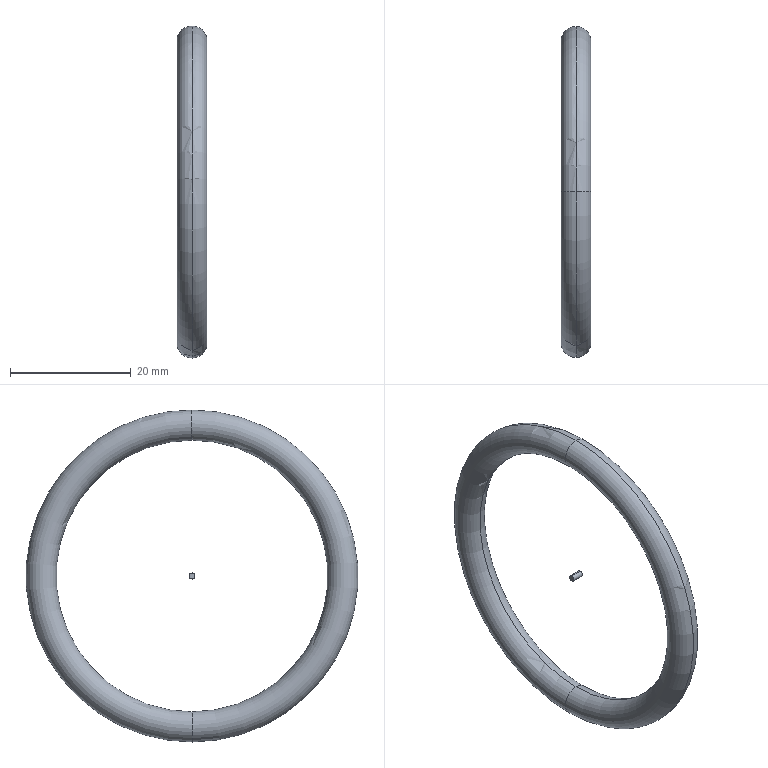Part | STEP file | Tension spring | 2 solids | 12 faces | box 5 x 55 x 55 mm | volume 1304 mm3 | torus 8 | cylinder 2 | plane 2 | commonest cylinder face diameters 1 x2
STEP:
#1=CARTESIAN_POINT('',(0.,0.,0.));
#2=DIRECTION('',(0.,0.,1.));
#3=DIRECTION('',(1.,0.,0.));
#4=AXIS2_PLACEMENT_3D('',#1,#2,#3);
#5=CARTESIAN_POINT('',(0.,0.,2.5));
#6=VERTEX_POINT('',#5);
#7=CARTESIAN_POINT('',(0.,0.,-2.5));
#8=VERTEX_POINT('',#7);
#9=CARTESIAN_POINT('',(0.,0.,0.));
#10=DIRECTION('',(0.,1.,0.));
#11=DIRECTION('',(0.,0.,1.));
#12=AXIS2_PLACEMENT_3D('',#9,#10,#11);
#13=CIRCLE('',#12,2.5);
#14=CARTESIAN_POINT('',(0.,0.,-25.));
#15=DIRECTION('',(1.,0.,0.));
#16=DIRECTION('',(0.,0.,-1.));
#17=AXIS2_PLACEMENT_3D('',#14,#15,#16);
#18=TOROIDAL_SURFACE('',#17,25.,2.5);
#19=CARTESIAN_POINT('',(3.142,0.));
#20=DIRECTION('',(0.,1.));
#21=VECTOR('',#20,1.);
#22=LINE('',#19,#21);
#23=(GEOMETRIC_REPRESENTATION_CONTEXT(2)PARAMETRIC_REPRESENTATION_CONTEXT()REPRESENTATION_CONTEXT('',''));
#24=DEFINITIONAL_REPRESENTATION('',(#22),#23);
#25=PCURVE('',#18,#24);
#26=CARTESIAN_POINT('',(0.,0.,-25.));
#27=DIRECTION('',(1.,0.,0.));
#28=DIRECTION('',(0.,0.,-1.));
#29=AXIS2_PLACEMENT_3D('',#26,#27,#28);
#30=TOROIDAL_SURFACE('',#29,25.,2.5);
#31=CARTESIAN_POINT('',(3.142,0.));
#32=DIRECTION('',(0.,1.));
#33=VECTOR('',#32,1.);
#34=LINE('',#31,#33);
#35=(GEOMETRIC_REPRESENTATION_CONTEXT(2)PARAMETRIC_REPRESENTATION_CONTEXT()REPRESENTATION_CONTEXT('',''));
#36=DEFINITIONAL_REPRESENTATION('',(#34),#35);
#37=PCURVE('',#30,#36);
#38=SURFACE_CURVE('',#13,(#25,#37),.PCURVE_S1.);
#39=EDGE_CURVE('',#6,#8,#38,.T.);
#40=ORIENTED_EDGE('',*,*,#39,.F.);
#41=CARTESIAN_POINT('',(0.,0.,-52.5));
#42=VERTEX_POINT('',#41);
#43=CARTESIAN_POINT('',(0.,0.,-25.));
#44=DIRECTION('',(1.,0.,0.));
#45=DIRECTION('',(0.,0.,-1.));
#46=AXIS2_PLACEMENT_3D('',#43,#44,#45);
#47=CIRCLE('',#46,27.5);
#48=CARTESIAN_POINT('',(0.,0.));
#49=DIRECTION('',(1.,0.));
#50=VECTOR('',#49,1.);
#51=LINE('',#48,#50);
#52=(GEOMETRIC_REPRESENTATION_CONTEXT(2)PARAMETRIC_REPRESENTATION_CONTEXT()REPRESENTATION_CONTEXT('',''));
#53=DEFINITIONAL_REPRESENTATION('',(#51),#52);
#54=PCURVE('',#18,#53);
#55=CARTESIAN_POINT('',(0.,0.,-25.));
#56=DIRECTION('',(1.,0.,0.));
#57=DIRECTION('',(0.,0.,-1.));
#58=AXIS2_PLACEMENT_3D('',#55,#56,#57);
#59=TOROIDAL_SURFACE('',#58,25.,2.5);
#60=CARTESIAN_POINT('',(0.,6.283));
#61=DIRECTION('',(1.,0.));
#62=VECTOR('',#61,1.);
#63=LINE('',#60,#62);
#64=(GEOMETRIC_REPRESENTATION_CONTEXT(2)PARAMETRIC_REPRESENTATION_CONTEXT()REPRESENTATION_CONTEXT('',''));
#65=DEFINITIONAL_REPRESENTATION('',(#63),#64);
#66=PCURVE('',#59,#65);
#67=SURFACE_CURVE('',#47,(#54,#66),.PCURVE_S1.);
#68=EDGE_CURVE('',#6,#42,#67,.T.);
#69=ORIENTED_EDGE('',*,*,#68,.T.);
#70=CARTESIAN_POINT('',(0.,0.,-47.5));
#71=VERTEX_POINT('',#70);
#72=CARTESIAN_POINT('',(0.,0.,-50.));
#73=DIRECTION('',(0.,-1.,0.));
#74=DIRECTION('',(0.,0.,-1.));
#75=AXIS2_PLACEMENT_3D('',#72,#73,#74);
#76=CIRCLE('',#75,2.5);
#77=CARTESIAN_POINT('',(6.283,0.));
#78=DIRECTION('',(0.,1.));
#79=VECTOR('',#78,1.);
#80=LINE('',#77,#79);
#81=(GEOMETRIC_REPRESENTATION_CONTEXT(2)PARAMETRIC_REPRESENTATION_CONTEXT()REPRESENTATION_CONTEXT('',''));
#82=DEFINITIONAL_REPRESENTATION('',(#80),#81);
#83=PCURVE('',#18,#82);
#84=CARTESIAN_POINT('',(0.,0.));
#85=DIRECTION('',(0.,1.));
#86=VECTOR('',#85,1.);
#87=LINE('',#84,#86);
#88=(GEOMETRIC_REPRESENTATION_CONTEXT(2)PARAMETRIC_REPRESENTATION_CONTEXT()REPRESENTATION_CONTEXT('',''));
#89=DEFINITIONAL_REPRESENTATION('',(#87),#88);
#90=PCURVE('',#30,#89);
#91=SURFACE_CURVE('',#76,(#83,#90),.PCURVE_S1.);
#92=EDGE_CURVE('',#42,#71,#91,.T.);
#93=ORIENTED_EDGE('',*,*,#92,.T.);
#94=CARTESIAN_POINT('',(0.,0.,-25.));
#95=DIRECTION('',(1.,0.,0.));
#96=DIRECTION('',(0.,0.,-1.));
#97=AXIS2_PLACEMENT_3D('',#94,#95,#96);
#98=CIRCLE('',#97,22.5);
#99=CARTESIAN_POINT('',(0.,3.142));
#100=DIRECTION('',(1.,0.));
#101=VECTOR('',#100,1.);
#102=LINE('',#99,#101);
#103=(GEOMETRIC_REPRESENTATION_CONTEXT(2)PARAMETRIC_REPRESENTATION_CONTEXT()REPRESENTATION_CONTEXT('',''));
#104=DEFINITIONAL_REPRESENTATION('',(#102),#103);
#105=PCURVE('',#18,#104);
#106=CARTESIAN_POINT('',(0.,3.142));
#107=DIRECTION('',(1.,0.));
#108=VECTOR('',#107,1.);
#109=LINE('',#106,#108);
#110=(GEOMETRIC_REPRESENTATION_CONTEXT(2)PARAMETRIC_REPRESENTATION_CONTEXT()REPRESENTATION_CONTEXT('',''));
#111=DEFINITIONAL_REPRESENTATION('',(#109),#110);
#112=PCURVE('',#59,#111);
#113=SURFACE_CURVE('',#98,(#105,#112),.PCURVE_S1.);
#114=EDGE_CURVE('',#8,#71,#113,.T.);
#115=ORIENTED_EDGE('',*,*,#114,.F.);
#116=EDGE_LOOP('',(#40,#69,#93,#115));
#117=FACE_BOUND('',#116,.T.);
#118=ADVANCED_FACE('',(#117),#18,.T.);
#119=ORIENTED_EDGE('',*,*,#92,.F.);
#120=CARTESIAN_POINT('',(0.,0.,-25.));
#121=DIRECTION('',(1.,0.,0.));
#122=DIRECTION('',(0.,0.,-1.));
#123=AXIS2_PLACEMENT_3D('',#120,#121,#122);
#124=CIRCLE('',#123,27.5);
#125=CARTESIAN_POINT('',(0.,0.));
#126=DIRECTION('',(1.,0.));
#127=VECTOR('',#126,1.);
#128=LINE('',#125,#127);
#129=(GEOMETRIC_REPRESENTATION_CONTEXT(2)PARAMETRIC_REPRESENTATION_CONTEXT()REPRESENTATION_CONTEXT('',''));
#130=DEFINITIONAL_REPRESENTATION('',(#128),#129);
#131=PCURVE('',#30,#130);
#132=CARTESIAN_POINT('',(0.,0.,-25.));
#133=DIRECTION('',(1.,0.,0.));
#134=DIRECTION('',(0.,0.,-1.));
#135=AXIS2_PLACEMENT_3D('',#132,#133,#134);
#136=TOROIDAL_SURFACE('',#135,25.,2.5);
#137=CARTESIAN_POINT('',(0.,6.283));
#138=DIRECTION('',(1.,0.));
#139=VECTOR('',#138,1.);
#140=LINE('',#137,#139);
#141=(GEOMETRIC_REPRESENTATION_CONTEXT(2)PARAMETRIC_REPRESENTATION_CONTEXT()REPRESENTATION_CONTEXT('',''));
#142=DEFINITIONAL_REPRESENTATION('',(#140),#141);
#143=PCURVE('',#136,#142);
#144=SURFACE_CURVE('',#124,(#131,#143),.PCURVE_S1.);
#145=EDGE_CURVE('',#42,#6,#144,.T.);
#146=ORIENTED_EDGE('',*,*,#145,.T.);
#147=ORIENTED_EDGE('',*,*,#39,.T.);
#148=CARTESIAN_POINT('',(0.,0.,-25.));
#149=DIRECTION('',(1.,0.,0.));
#150=DIRECTION('',(0.,0.,-1.));
#151=AXIS2_PLACEMENT_3D('',#148,#149,#150);
#152=CIRCLE('',#151,22.5);
#153=CARTESIAN_POINT('',(0.,3.142));
#154=DIRECTION('',(1.,0.));
#155=VECTOR('',#154,1.);
#156=LINE('',#153,#155);
#157=(GEOMETRIC_REPRESENTATION_CONTEXT(2)PARAMETRIC_REPRESENTATION_CONTEXT()REPRESENTATION_CONTEXT('',''));
#158=DEFINITIONAL_REPRESENTATION('',(#156),#157);
#159=PCURVE('',#30,#158);
#160=CARTESIAN_POINT('',(0.,3.142));
#161=DIRECTION('',(1.,0.));
#162=VECTOR('',#161,1.);
#163=LINE('',#160,#162);
#164=(GEOMETRIC_REPRESENTATION_CONTEXT(2)PARAMETRIC_REPRESENTATION_CONTEXT()REPRESENTATION_CONTEXT('',''));
#165=DEFINITIONAL_REPRESENTATION('',(#163),#164);
#166=PCURVE('',#136,#165);
#167=SURFACE_CURVE('',#152,(#159,#166),.PCURVE_S1.);
#168=EDGE_CURVE('',#71,#8,#167,.T.);
#169=ORIENTED_EDGE('',*,*,#168,.F.);
#170=EDGE_LOOP('',(#119,#146,#147,#169));
#171=FACE_BOUND('',#170,.T.);
#172=ADVANCED_FACE('',(#171),#30,.T.);
#173=ORIENTED_EDGE('',*,*,#145,.F.);
#174=CARTESIAN_POINT('',(0.,0.,-50.));
#175=DIRECTION('',(0.,-1.,0.));
#176=DIRECTION('',(0.,0.,-1.));
#177=AXIS2_PLACEMENT_3D('',#174,#175,#176);
#178=CIRCLE('',#177,2.5);
#179=CARTESIAN_POINT('',(0.,0.));
#180=DIRECTION('',(0.,1.));
#181=VECTOR('',#180,1.);
#182=LINE('',#179,#181);
#183=(GEOMETRIC_REPRESENTATION_CONTEXT(2)PARAMETRIC_REPRESENTATION_CONTEXT()REPRESENTATION_CONTEXT('',''));
#184=DEFINITIONAL_REPRESENTATION('',(#182),#183);
#185=PCURVE('',#136,#184);
#186=CARTESIAN_POINT('',(6.283,0.));
#187=DIRECTION('',(0.,1.));
#188=VECTOR('',#187,1.);
#189=LINE('',#186,#188);
#190=(GEOMETRIC_REPRESENTATION_CONTEXT(2)PARAMETRIC_REPRESENTATION_CONTEXT()REPRESENTATION_CONTEXT('',''));
#191=DEFINITIONAL_REPRESENTATION('',(#189),#190);
#192=PCURVE('',#59,#191);
#193=SURFACE_CURVE('',#178,(#185,#192),.PCURVE_S1.);
#194=EDGE_CURVE('',#71,#42,#193,.T.);
#195=ORIENTED_EDGE('',*,*,#194,.F.);
#196=ORIENTED_EDGE('',*,*,#168,.T.);
#197=CARTESIAN_POINT('',(0.,0.,0.));
#198=DIRECTION('',(0.,1.,0.));
#199=DIRECTION('',(0.,0.,1.));
#200=AXIS2_PLACEMENT_3D('',#197,#198,#199);
#201=CIRCLE('',#200,2.5);
#202=CARTESIAN_POINT('',(3.142,0.));
#203=DIRECTION('',(0.,1.));
#204=VECTOR('',#203,1.);
#205=LINE('',#202,#204);
#206=(GEOMETRIC_REPRESENTATION_CONTEXT(2)PARAMETRIC_REPRESENTATION_CONTEXT()REPRESENTATION_CONTEXT('',''));
#207=DEFINITIONAL_REPRESENTATION('',(#205),#206);
#208=PCURVE('',#136,#207);
#209=CARTESIAN_POINT('',(3.142,0.));
#210=DIRECTION('',(0.,1.));
#211=VECTOR('',#210,1.);
#212=LINE('',#209,#211);
#213=(GEOMETRIC_REPRESENTATION_CONTEXT(2)PARAMETRIC_REPRESENTATION_CONTEXT()REPRESENTATION_CONTEXT('',''));
#214=DEFINITIONAL_REPRESENTATION('',(#212),#213);
#215=PCURVE('',#59,#214);
#216=SURFACE_CURVE('',#201,(#208,#215),.PCURVE_S1.);
#217=EDGE_CURVE('',#8,#6,#216,.T.);
#218=ORIENTED_EDGE('',*,*,#217,.T.);
#219=EDGE_LOOP('',(#173,#195,#196,#218));
#220=FACE_BOUND('',#219,.T.);
#221=ADVANCED_FACE('',(#220),#136,.T.);
#222=ORIENTED_EDGE('',*,*,#68,.F.);
#223=ORIENTED_EDGE('',*,*,#217,.F.);
#224=ORIENTED_EDGE('',*,*,#114,.T.);
#225=ORIENTED_EDGE('',*,*,#194,.T.);
#226=EDGE_LOOP('',(#222,#223,#224,#225));
#227=FACE_BOUND('',#226,.T.);
#228=ADVANCED_FACE('',(#227),#59,.T.);
#229=CLOSED_SHELL('',(#118,#172,#221,#228));
#230=CARTESIAN_POINT('',(0.,0.,-48.1));
#231=VERTEX_POINT('',#230);
#232=CARTESIAN_POINT('',(0.,0.,-1.9));
#233=VERTEX_POINT('',#232);
#234=CARTESIAN_POINT('',(0.,0.,-25.));
#235=DIRECTION('',(1.,0.,0.));
#236=DIRECTION('',(0.,0.,-1.));
#237=AXIS2_PLACEMENT_3D('',#234,#235,#236);
#238=CIRCLE('',#237,23.1);
#239=CARTESIAN_POINT('',(0.,0.,-25.));
#240=DIRECTION('',(1.,0.,0.));
#241=DIRECTION('',(0.,0.,-1.));
#242=AXIS2_PLACEMENT_3D('',#239,#240,#241);
#243=TOROIDAL_SURFACE('',#242,25.,1.9);
#244=CARTESIAN_POINT('',(0.,3.142));
#245=DIRECTION('',(1.,0.));
#246=VECTOR('',#245,1.);
#247=LINE('',#244,#246);
#248=(GEOMETRIC_REPRESENTATION_CONTEXT(2)PARAMETRIC_REPRESENTATION_CONTEXT()REPRESENTATION_CONTEXT('',''));
#249=DEFINITIONAL_REPRESENTATION('',(#247),#248);
#250=PCURVE('',#243,#249);
#251=CARTESIAN_POINT('',(0.,0.,-25.));
#252=DIRECTION('',(1.,0.,0.));
#253=DIRECTION('',(0.,0.,-1.));
#254=AXIS2_PLACEMENT_3D('',#251,#252,#253);
#255=TOROIDAL_SURFACE('',#254,25.,1.9);
#256=CARTESIAN_POINT('',(0.,3.142));
#257=DIRECTION('',(1.,0.));
#258=VECTOR('',#257,1.);
#259=LINE('',#256,#258);
#260=(GEOMETRIC_REPRESENTATION_CONTEXT(2)PARAMETRIC_REPRESENTATION_CONTEXT()REPRESENTATION_CONTEXT('',''));
#261=DEFINITIONAL_REPRESENTATION('',(#259),#260);
#262=PCURVE('',#255,#261);
#263=SURFACE_CURVE('',#238,(#250,#262),.PCURVE_S1.);
#264=EDGE_CURVE('',#231,#233,#263,.T.);
#265=ORIENTED_EDGE('',*,*,#264,.T.);
#266=CARTESIAN_POINT('',(0.,0.,1.9));
#267=VERTEX_POINT('',#266);
#268=CARTESIAN_POINT('',(0.,0.,0.));
#269=DIRECTION('',(0.,1.,0.));
#270=DIRECTION('',(0.,0.,1.));
#271=AXIS2_PLACEMENT_3D('',#268,#269,#270);
#272=CIRCLE('',#271,1.9);
#273=CARTESIAN_POINT('',(3.142,0.));
#274=DIRECTION('',(0.,1.));
#275=VECTOR('',#274,1.);
#276=LINE('',#273,#275);
#277=(GEOMETRIC_REPRESENTATION_CONTEXT(2)PARAMETRIC_REPRESENTATION_CONTEXT()REPRESENTATION_CONTEXT('',''));
#278=DEFINITIONAL_REPRESENTATION('',(#276),#277);
#279=PCURVE('',#243,#278);
#280=CARTESIAN_POINT('',(0.,0.,-25.));
#281=DIRECTION('',(1.,0.,0.));
#282=DIRECTION('',(0.,0.,-1.));
#283=AXIS2_PLACEMENT_3D('',#280,#281,#282);
#284=TOROIDAL_SURFACE('',#283,25.,1.9);
#285=CARTESIAN_POINT('',(3.142,0.));
#286=DIRECTION('',(0.,1.));
#287=VECTOR('',#286,1.);
#288=LINE('',#285,#287);
#289=(GEOMETRIC_REPRESENTATION_CONTEXT(2)PARAMETRIC_REPRESENTATION_CONTEXT()REPRESENTATION_CONTEXT('',''));
#290=DEFINITIONAL_REPRESENTATION('',(#288),#289);
#291=PCURVE('',#284,#290);
#292=SURFACE_CURVE('',#272,(#279,#291),.PCURVE_S1.);
#293=EDGE_CURVE('',#233,#267,#292,.T.);
#294=ORIENTED_EDGE('',*,*,#293,.T.);
#295=CARTESIAN_POINT('',(0.,0.,-51.9));
#296=VERTEX_POINT('',#295);
#297=CARTESIAN_POINT('',(0.,0.,-25.));
#298=DIRECTION('',(1.,0.,0.));
#299=DIRECTION('',(0.,0.,-1.));
#300=AXIS2_PLACEMENT_3D('',#297,#298,#299);
#301=CIRCLE('',#300,26.9);
#302=CARTESIAN_POINT('',(0.,6.283));
#303=DIRECTION('',(1.,0.));
#304=VECTOR('',#303,1.);
#305=LINE('',#302,#304);
#306=(GEOMETRIC_REPRESENTATION_CONTEXT(2)PARAMETRIC_REPRESENTATION_CONTEXT()REPRESENTATION_CONTEXT('',''));
#307=DEFINITIONAL_REPRESENTATION('',(#305),#306);
#308=PCURVE('',#243,#307);
#309=CARTESIAN_POINT('',(0.,0.));
#310=DIRECTION('',(1.,0.));
#311=VECTOR('',#310,1.);
#312=LINE('',#309,#311);
#313=(GEOMETRIC_REPRESENTATION_CONTEXT(2)PARAMETRIC_REPRESENTATION_CONTEXT()REPRESENTATION_CONTEXT('',''));
#314=DEFINITIONAL_REPRESENTATION('',(#312),#313);
#315=PCURVE('',#255,#314);
#316=SURFACE_CURVE('',#301,(#308,#315),.PCURVE_S1.);
#317=EDGE_CURVE('',#296,#267,#316,.T.);
#318=ORIENTED_EDGE('',*,*,#317,.F.);
#319=CARTESIAN_POINT('',(0.,0.,-50.));
#320=DIRECTION('',(0.,-1.,0.));
#321=DIRECTION('',(0.,0.,-1.));
#322=AXIS2_PLACEMENT_3D('',#319,#320,#321);
#323=CIRCLE('',#322,1.9);
#324=CARTESIAN_POINT('',(0.,0.));
#325=DIRECTION('',(0.,1.));
#326=VECTOR('',#325,1.);
#327=LINE('',#324,#326);
#328=(GEOMETRIC_REPRESENTATION_CONTEXT(2)PARAMETRIC_REPRESENTATION_CONTEXT()REPRESENTATION_CONTEXT('',''));
#329=DEFINITIONAL_REPRESENTATION('',(#327),#328);
#330=PCURVE('',#243,#329);
#331=CARTESIAN_POINT('',(6.283,0.));
#332=DIRECTION('',(0.,1.));
#333=VECTOR('',#332,1.);
#334=LINE('',#331,#333);
#335=(GEOMETRIC_REPRESENTATION_CONTEXT(2)PARAMETRIC_REPRESENTATION_CONTEXT()REPRESENTATION_CONTEXT('',''));
#336=DEFINITIONAL_REPRESENTATION('',(#334),#335);
#337=PCURVE('',#284,#336);
#338=SURFACE_CURVE('',#323,(#330,#337),.PCURVE_S1.);
#339=EDGE_CURVE('',#231,#296,#338,.T.);
#340=ORIENTED_EDGE('',*,*,#339,.F.);
#341=EDGE_LOOP('',(#265,#294,#318,#340));
#342=FACE_BOUND('',#341,.T.);
#343=ADVANCED_FACE('',(#342),#243,.T.);
#344=CARTESIAN_POINT('',(0.,0.,-25.));
#345=DIRECTION('',(1.,0.,0.));
#346=DIRECTION('',(0.,0.,-1.));
#347=AXIS2_PLACEMENT_3D('',#344,#345,#346);
#348=CIRCLE('',#347,23.1);
#349=CARTESIAN_POINT('',(0.,3.142));
#350=DIRECTION('',(1.,0.));
#351=VECTOR('',#350,1.);
#352=LINE('',#349,#351);
#353=(GEOMETRIC_REPRESENTATION_CONTEXT(2)PARAMETRIC_REPRESENTATION_CONTEXT()REPRESENTATION_CONTEXT('',''));
#354=DEFINITIONAL_REPRESENTATION('',(#352),#353);
#355=PCURVE('',#284,#354);
#356=CARTESIAN_POINT('',(0.,0.,-25.));
#357=DIRECTION('',(1.,0.,0.));
#358=DIRECTION('',(0.,0.,-1.));
#359=AXIS2_PLACEMENT_3D('',#356,#357,#358);
#360=TOROIDAL_SURFACE('',#359,25.,1.9);
#361=CARTESIAN_POINT('',(0.,3.142));
#362=DIRECTION('',(1.,0.));
#363=VECTOR('',#362,1.);
#364=LINE('',#361,#363);
#365=(GEOMETRIC_REPRESENTATION_CONTEXT(2)PARAMETRIC_REPRESENTATION_CONTEXT()REPRESENTATION_CONTEXT('',''));
#366=DEFINITIONAL_REPRESENTATION('',(#364),#365);
#367=PCURVE('',#360,#366);
#368=SURFACE_CURVE('',#348,(#355,#367),.PCURVE_S1.);
#369=EDGE_CURVE('',#233,#231,#368,.T.);
#370=ORIENTED_EDGE('',*,*,#369,.T.);
#371=ORIENTED_EDGE('',*,*,#339,.T.);
#372=CARTESIAN_POINT('',(0.,0.,-25.));
#373=DIRECTION('',(1.,0.,0.));
#374=DIRECTION('',(0.,0.,-1.));
#375=AXIS2_PLACEMENT_3D('',#372,#373,#374);
#376=CIRCLE('',#375,26.9);
#377=CARTESIAN_POINT('',(0.,6.283));
#378=DIRECTION('',(1.,0.));
#379=VECTOR('',#378,1.);
#380=LINE('',#377,#379);
#381=(GEOMETRIC_REPRESENTATION_CONTEXT(2)PARAMETRIC_REPRESENTATION_CONTEXT()REPRESENTATION_CONTEXT('',''));
#382=DEFINITIONAL_REPRESENTATION('',(#380),#381);
#383=PCURVE('',#284,#382);
#384=CARTESIAN_POINT('',(0.,0.));
#385=DIRECTION('',(1.,0.));
#386=VECTOR('',#385,1.);
#387=LINE('',#384,#386);
#388=(GEOMETRIC_REPRESENTATION_CONTEXT(2)PARAMETRIC_REPRESENTATION_CONTEXT()REPRESENTATION_CONTEXT('',''));
#389=DEFINITIONAL_REPRESENTATION('',(#387),#388);
#390=PCURVE('',#360,#389);
#391=SURFACE_CURVE('',#376,(#383,#390),.PCURVE_S1.);
#392=EDGE_CURVE('',#267,#296,#391,.T.);
#393=ORIENTED_EDGE('',*,*,#392,.F.);
#394=ORIENTED_EDGE('',*,*,#293,.F.);
#395=EDGE_LOOP('',(#370,#371,#393,#394));
#396=FACE_BOUND('',#395,.T.);
#397=ADVANCED_FACE('',(#396),#284,.T.);
#398=CARTESIAN_POINT('',(0.,0.,-50.));
#399=DIRECTION('',(0.,-1.,0.));
#400=DIRECTION('',(0.,0.,-1.));
#401=AXIS2_PLACEMENT_3D('',#398,#399,#400);
#402=CIRCLE('',#401,1.9);
#403=CARTESIAN_POINT('',(6.283,0.));
#404=DIRECTION('',(0.,1.));
#405=VECTOR('',#404,1.);
#406=LINE('',#403,#405);
#407=(GEOMETRIC_REPRESENTATION_CONTEXT(2)PARAMETRIC_REPRESENTATION_CONTEXT()REPRESENTATION_CONTEXT('',''));
#408=DEFINITIONAL_REPRESENTATION('',(#406),#407);
#409=PCURVE('',#360,#408);
#410=CARTESIAN_POINT('',(0.,0.));
#411=DIRECTION('',(0.,1.));
#412=VECTOR('',#411,1.);
#413=LINE('',#410,#412);
#414=(GEOMETRIC_REPRESENTATION_CONTEXT(2)PARAMETRIC_REPRESENTATION_CONTEXT()REPRESENTATION_CONTEXT('',''));
#415=DEFINITIONAL_REPRESENTATION('',(#413),#414);
#416=PCURVE('',#255,#415);
#417=SURFACE_CURVE('',#402,(#409,#416),.PCURVE_S1.);
#418=EDGE_CURVE('',#296,#231,#417,.T.);
#419=ORIENTED_EDGE('',*,*,#418,.T.);
#420=ORIENTED_EDGE('',*,*,#369,.F.);
#421=CARTESIAN_POINT('',(0.,0.,0.));
#422=DIRECTION('',(0.,1.,0.));
#423=DIRECTION('',(0.,0.,1.));
#424=AXIS2_PLACEMENT_3D('',#421,#422,#423);
#425=CIRCLE('',#424,1.9);
#426=CARTESIAN_POINT('',(3.142,0.));
#427=DIRECTION('',(0.,1.));
#428=VECTOR('',#427,1.);
#429=LINE('',#426,#428);
#430=(GEOMETRIC_REPRESENTATION_CONTEXT(2)PARAMETRIC_REPRESENTATION_CONTEXT()REPRESENTATION_CONTEXT('',''));
#431=DEFINITIONAL_REPRESENTATION('',(#429),#430);
#432=PCURVE('',#360,#431);
#433=CARTESIAN_POINT('',(3.142,0.));
#434=DIRECTION('',(0.,1.));
#435=VECTOR('',#434,1.);
#436=LINE('',#433,#435);
#437=(GEOMETRIC_REPRESENTATION_CONTEXT(2)PARAMETRIC_REPRESENTATION_CONTEXT()REPRESENTATION_CONTEXT('',''));
#438=DEFINITIONAL_REPRESENTATION('',(#436),#437);
#439=PCURVE('',#255,#438);
#440=SURFACE_CURVE('',#425,(#432,#439),.PCURVE_S1.);
#441=EDGE_CURVE('',#267,#233,#440,.T.);
#442=ORIENTED_EDGE('',*,*,#441,.F.);
#443=ORIENTED_EDGE('',*,*,#392,.T.);
#444=EDGE_LOOP('',(#419,#420,#442,#443));
#445=FACE_BOUND('',#444,.T.);
#446=ADVANCED_FACE('',(#445),#360,.T.);
#447=ORIENTED_EDGE('',*,*,#441,.T.);
#448=ORIENTED_EDGE('',*,*,#264,.F.);
#449=ORIENTED_EDGE('',*,*,#418,.F.);
#450=ORIENTED_EDGE('',*,*,#317,.T.);
#451=EDGE_LOOP('',(#447,#448,#449,#450));
#452=FACE_BOUND('',#451,.T.);
#453=ADVANCED_FACE('',(#452),#255,.T.);
#454=CLOSED_SHELL('',(#343,#397,#446,#453));
#455=ORIENTED_CLOSED_SHELL('',*,#454,.F.);
#456=BREP_WITH_VOIDS('',#229,(#455));
#457=CARTESIAN_POINT('',(1.,0.,-25.5));
#458=VERTEX_POINT('',#457);
#459=CARTESIAN_POINT('',(1.,0.,-24.5));
#460=VERTEX_POINT('',#459);
#461=CARTESIAN_POINT('',(1.,0.,-25.));
#462=DIRECTION('',(1.,0.,0.));
#463=DIRECTION('',(0.,0.,-1.));
#464=AXIS2_PLACEMENT_3D('',#461,#462,#463);
#465=CIRCLE('',#464,0.5);
#466=CARTESIAN_POINT('',(1.,0.,-25.));
#467=DIRECTION('',(-1.,0.,0.));
#468=DIRECTION('',(0.,0.,1.));
#469=AXIS2_PLACEMENT_3D('',#466,#467,#468);
#470=CYLINDRICAL_SURFACE('',#469,0.5);
#471=CARTESIAN_POINT('',(3.142,0.));
#472=DIRECTION('',(-1.,0.));
#473=VECTOR('',#472,1.);
#474=LINE('',#471,#473);
#475=(GEOMETRIC_REPRESENTATION_CONTEXT(2)PARAMETRIC_REPRESENTATION_CONTEXT()REPRESENTATION_CONTEXT('',''));
#476=DEFINITIONAL_REPRESENTATION('',(#474),#475);
#477=PCURVE('',#470,#476);
#478=CARTESIAN_POINT('',(1.,0.,-25.));
#479=DIRECTION('',(1.,0.,0.));
#480=DIRECTION('',(0.,0.,-1.));
#481=AXIS2_PLACEMENT_3D('',#478,#479,#480);
#482=PLANE('',#481);
#483=CARTESIAN_POINT('',(0.,0.));
#484=DIRECTION('',(1.,0.));
#485=AXIS2_PLACEMENT_2D('',#483,#484);
#486=CIRCLE('',#485,0.5);
#487=(GEOMETRIC_REPRESENTATION_CONTEXT(2)PARAMETRIC_REPRESENTATION_CONTEXT()REPRESENTATION_CONTEXT('',''));
#488=DEFINITIONAL_REPRESENTATION('',(#486),#487);
#489=PCURVE('',#482,#488);
#490=SURFACE_CURVE('',#465,(#477,#489),.PCURVE_S1.);
#491=EDGE_CURVE('',#458,#460,#490,.T.);
#492=ORIENTED_EDGE('',*,*,#491,.F.);
#493=CARTESIAN_POINT('',(-1.,0.,-25.5));
#494=VERTEX_POINT('',#493);
#495=CARTESIAN_POINT('',(1.,0.,-25.5));
#496=DIRECTION('',(-1.,0.,0.));
#497=VECTOR('',#496,1.);
#498=LINE('',#495,#497);
#499=CARTESIAN_POINT('',(3.142,0.));
#500=DIRECTION('',(0.,1.));
#501=VECTOR('',#500,1.);
#502=LINE('',#499,#501);
#503=(GEOMETRIC_REPRESENTATION_CONTEXT(2)PARAMETRIC_REPRESENTATION_CONTEXT()REPRESENTATION_CONTEXT('',''));
#504=DEFINITIONAL_REPRESENTATION('',(#502),#503);
#505=PCURVE('',#470,#504);
#506=CARTESIAN_POINT('',(1.,0.,-25.));
#507=DIRECTION('',(-1.,0.,0.));
#508=DIRECTION('',(0.,0.,1.));
#509=AXIS2_PLACEMENT_3D('',#506,#507,#508);
#510=CYLINDRICAL_SURFACE('',#509,0.5);
#511=CARTESIAN_POINT('',(3.142,0.));
#512=DIRECTION('',(0.,1.));
#513=VECTOR('',#512,1.);
#514=LINE('',#511,#513);
#515=(GEOMETRIC_REPRESENTATION_CONTEXT(2)PARAMETRIC_REPRESENTATION_CONTEXT()REPRESENTATION_CONTEXT('',''));
#516=DEFINITIONAL_REPRESENTATION('',(#514),#515);
#517=PCURVE('',#510,#516);
#518=SURFACE_CURVE('',#498,(#505,#517),.PCURVE_S1.);
#519=EDGE_CURVE('',#458,#494,#518,.T.);
#520=ORIENTED_EDGE('',*,*,#519,.T.);
#521=CARTESIAN_POINT('',(-1.,0.,-24.5));
#522=VERTEX_POINT('',#521);
#523=CARTESIAN_POINT('',(-1.,0.,-25.));
#524=DIRECTION('',(1.,0.,0.));
#525=DIRECTION('',(0.,0.,-1.));
#526=AXIS2_PLACEMENT_3D('',#523,#524,#525);
#527=CIRCLE('',#526,0.5);
#528=CARTESIAN_POINT('',(3.142,2.));
#529=DIRECTION('',(-1.,0.));
#530=VECTOR('',#529,1.);
#531=LINE('',#528,#530);
#532=(GEOMETRIC_REPRESENTATION_CONTEXT(2)PARAMETRIC_REPRESENTATION_CONTEXT()REPRESENTATION_CONTEXT('',''));
#533=DEFINITIONAL_REPRESENTATION('',(#531),#532);
#534=PCURVE('',#470,#533);
#535=CARTESIAN_POINT('',(-1.,0.,-25.));
#536=DIRECTION('',(1.,0.,0.));
#537=DIRECTION('',(0.,0.,-1.));
#538=AXIS2_PLACEMENT_3D('',#535,#536,#537);
#539=PLANE('',#538);
#540=CARTESIAN_POINT('',(0.,0.));
#541=DIRECTION('',(1.,0.));
#542=AXIS2_PLACEMENT_2D('',#540,#541);
#543=CIRCLE('',#542,0.5);
#544=(GEOMETRIC_REPRESENTATION_CONTEXT(2)PARAMETRIC_REPRESENTATION_CONTEXT()REPRESENTATION_CONTEXT('',''));
#545=DEFINITIONAL_REPRESENTATION('',(#543),#544);
#546=PCURVE('',#539,#545);
#547=SURFACE_CURVE('',#527,(#534,#546),.PCURVE_S1.);
#548=EDGE_CURVE('',#494,#522,#547,.T.);
#549=ORIENTED_EDGE('',*,*,#548,.T.);
#550=CARTESIAN_POINT('',(1.,0.,-24.5));
#551=DIRECTION('',(-1.,0.,0.));
#552=VECTOR('',#551,1.);
#553=LINE('',#550,#552);
#554=CARTESIAN_POINT('',(0.,0.));
#555=DIRECTION('',(0.,1.));
#556=VECTOR('',#555,1.);
#557=LINE('',#554,#556);
#558=(GEOMETRIC_REPRESENTATION_CONTEXT(2)PARAMETRIC_REPRESENTATION_CONTEXT()REPRESENTATION_CONTEXT('',''));
#559=DEFINITIONAL_REPRESENTATION('',(#557),#558);
#560=PCURVE('',#470,#559);
#561=CARTESIAN_POINT('',(6.283,0.));
#562=DIRECTION('',(0.,1.));
#563=VECTOR('',#562,1.);
#564=LINE('',#561,#563);
#565=(GEOMETRIC_REPRESENTATION_CONTEXT(2)PARAMETRIC_REPRESENTATION_CONTEXT()REPRESENTATION_CONTEXT('',''));
#566=DEFINITIONAL_REPRESENTATION('',(#564),#565);
#567=PCURVE('',#510,#566);
#568=SURFACE_CURVE('',#553,(#560,#567),.PCURVE_S1.);
#569=EDGE_CURVE('',#460,#522,#568,.T.);
#570=ORIENTED_EDGE('',*,*,#569,.F.);
#571=EDGE_LOOP('',(#492,#520,#549,#570));
#572=FACE_BOUND('',#571,.T.);
#573=ADVANCED_FACE('',(#572),#470,.T.);
#574=ORIENTED_EDGE('',*,*,#519,.F.);
#575=CARTESIAN_POINT('',(1.,0.,-25.));
#576=DIRECTION('',(1.,0.,0.));
#577=DIRECTION('',(0.,0.,-1.));
#578=AXIS2_PLACEMENT_3D('',#575,#576,#577);
#579=CIRCLE('',#578,0.5);
#580=CARTESIAN_POINT('',(9.425,0.));
#581=DIRECTION('',(-1.,0.));
#582=VECTOR('',#581,1.);
#583=LINE('',#580,#582);
#584=(GEOMETRIC_REPRESENTATION_CONTEXT(2)PARAMETRIC_REPRESENTATION_CONTEXT()REPRESENTATION_CONTEXT('',''));
#585=DEFINITIONAL_REPRESENTATION('',(#583),#584);
#586=PCURVE('',#510,#585);
#587=CARTESIAN_POINT('',(0.,0.));
#588=DIRECTION('',(1.,0.));
#589=AXIS2_PLACEMENT_2D('',#587,#588);
#590=CIRCLE('',#589,0.5);
#591=(GEOMETRIC_REPRESENTATION_CONTEXT(2)PARAMETRIC_REPRESENTATION_CONTEXT()REPRESENTATION_CONTEXT('',''));
#592=DEFINITIONAL_REPRESENTATION('',(#590),#591);
#593=PCURVE('',#482,#592);
#594=SURFACE_CURVE('',#579,(#586,#593),.PCURVE_S1.);
#595=EDGE_CURVE('',#460,#458,#594,.T.);
#596=ORIENTED_EDGE('',*,*,#595,.F.);
#597=ORIENTED_EDGE('',*,*,#569,.T.);
#598=CARTESIAN_POINT('',(-1.,0.,-25.));
#599=DIRECTION('',(1.,0.,0.));
#600=DIRECTION('',(0.,0.,-1.));
#601=AXIS2_PLACEMENT_3D('',#598,#599,#600);
#602=CIRCLE('',#601,0.5);
#603=CARTESIAN_POINT('',(9.425,2.));
#604=DIRECTION('',(-1.,0.));
#605=VECTOR('',#604,1.);
#606=LINE('',#603,#605);
#607=(GEOMETRIC_REPRESENTATION_CONTEXT(2)PARAMETRIC_REPRESENTATION_CONTEXT()REPRESENTATION_CONTEXT('',''));
#608=DEFINITIONAL_REPRESENTATION('',(#606),#607);
#609=PCURVE('',#510,#608);
#610=CARTESIAN_POINT('',(0.,0.));
#611=DIRECTION('',(1.,0.));
#612=AXIS2_PLACEMENT_2D('',#610,#611);
#613=CIRCLE('',#612,0.5);
#614=(GEOMETRIC_REPRESENTATION_CONTEXT(2)PARAMETRIC_REPRESENTATION_CONTEXT()REPRESENTATION_CONTEXT('',''));
#615=DEFINITIONAL_REPRESENTATION('',(#613),#614);
#616=PCURVE('',#539,#615);
#617=SURFACE_CURVE('',#602,(#609,#616),.PCURVE_S1.);
#618=EDGE_CURVE('',#522,#494,#617,.T.);
#619=ORIENTED_EDGE('',*,*,#618,.T.);
#620=EDGE_LOOP('',(#574,#596,#597,#619));
#621=FACE_BOUND('',#620,.T.);
#622=ADVANCED_FACE('',(#621),#510,.T.);
#623=ORIENTED_EDGE('',*,*,#595,.T.);
#624=ORIENTED_EDGE('',*,*,#491,.T.);
#625=EDGE_LOOP('',(#623,#624));
#626=FACE_BOUND('',#625,.T.);
#627=ADVANCED_FACE('',(#626),#482,.T.);
#628=ORIENTED_EDGE('',*,*,#618,.F.);
#629=ORIENTED_EDGE('',*,*,#548,.F.);
#630=EDGE_LOOP('',(#628,#629));
#631=FACE_BOUND('',#630,.T.);
#632=ADVANCED_FACE('',(#631),#539,.F.);
#633=CLOSED_SHELL('',(#573,#622,#627,#632));
#634=MANIFOLD_SOLID_BREP('',#633);
#635=(LENGTH_UNIT()NAMED_UNIT(*)SI_UNIT(.MILLI.,.METRE.));
#636=UNCERTAINTY_MEASURE_WITH_UNIT(LENGTH_MEASURE(0.0000001),#635,'','');
#637=(NAMED_UNIT(*)PLANE_ANGLE_UNIT()SI_UNIT($,.RADIAN.));
#638=(NAMED_UNIT(*)SI_UNIT($,.STERADIAN.)SOLID_ANGLE_UNIT());
#639=(GEOMETRIC_REPRESENTATION_CONTEXT(3)GLOBAL_UNCERTAINTY_ASSIGNED_CONTEXT((#636))GLOBAL_UNIT_ASSIGNED_CONTEXT((#635,#637,#638))REPRESENTATION_CONTEXT('',''));
#640=SHAPE_REPRESENTATION('',(#4,#456,#634),#639);